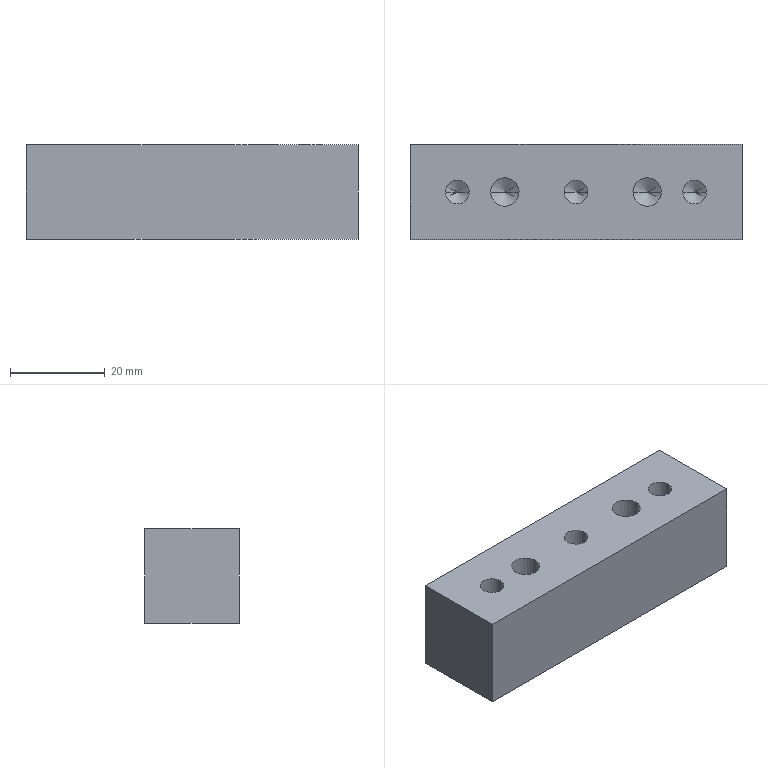Part | STEP file | 11-FG-B08711 | 1 solid | 26 faces | box 70 x 20 x 20 mm | volume 26205 mm3 | cylinder 10 | cone 10 | plane 6 | commonest cylinder face diameters 5 x6 6 x4
STEP:
#1=CARTESIAN_POINT('',(-18.,0.,5.));
#2=VERTEX_POINT('',#1);
#3=CARTESIAN_POINT('',(-12.,0.,5.));
#4=VERTEX_POINT('',#3);
#5=CARTESIAN_POINT('',(-15.,0.,5.));
#6=DIRECTION('',(0.,0.,1.));
#7=DIRECTION('',(1.,0.,0.));
#8=AXIS2_PLACEMENT_3D('',#5,#6,#7);
#9=CIRCLE('',#8,3.);
#10=EDGE_CURVE('',#2,#4,#9,.T.);
#11=ORIENTED_EDGE('',*,*,#10,.F.);
#12=CARTESIAN_POINT('',(-18.,0.,20.));
#13=VERTEX_POINT('',#12);
#14=CARTESIAN_POINT('',(-18.,0.,20.));
#15=DIRECTION('',(0.,0.,1.));
#16=VECTOR('',#15,1000.);
#17=LINE('',#14,#16);
#18=EDGE_CURVE('',#2,#13,#17,.T.);
#19=ORIENTED_EDGE('',*,*,#18,.T.);
#20=CARTESIAN_POINT('',(-12.,0.,20.));
#21=VERTEX_POINT('',#20);
#22=CARTESIAN_POINT('',(-15.,0.,20.));
#23=DIRECTION('',(0.,0.,1.));
#24=DIRECTION('',(1.,0.,0.));
#25=AXIS2_PLACEMENT_3D('',#22,#23,#24);
#26=CIRCLE('',#25,3.);
#27=EDGE_CURVE('',#13,#21,#26,.T.);
#28=ORIENTED_EDGE('',*,*,#27,.T.);
#29=CARTESIAN_POINT('',(-12.,0.,20.));
#30=DIRECTION('',(0.,0.,1.));
#31=VECTOR('',#30,1000.);
#32=LINE('',#29,#31);
#33=EDGE_CURVE('',#4,#21,#32,.T.);
#34=ORIENTED_EDGE('',*,*,#33,.F.);
#35=EDGE_LOOP('',(#11,#19,#28,#34));
#36=FACE_OUTER_BOUND('',#35,.T.);
#37=CARTESIAN_POINT('',(-15.,0.,20.));
#38=DIRECTION('',(0.,0.,1.));
#39=DIRECTION('',(1.,0.,0.));
#40=AXIS2_PLACEMENT_3D('',#37,#38,#39);
#41=CYLINDRICAL_SURFACE('',#40,3.);
#42=ADVANCED_FACE('',(#36),#41,.F.);
#43=CARTESIAN_POINT('',(-15.,0.,3.197));
#44=VERTEX_POINT('',#43);
#45=CARTESIAN_POINT('',(-12.,0.,5.));
#46=DIRECTION('',(0.8572,0.,0.515));
#47=VECTOR('',#46,1000.);
#48=LINE('',#45,#47);
#49=EDGE_CURVE('',#44,#4,#48,.T.);
#50=ORIENTED_EDGE('',*,*,#49,.F.);
#51=CARTESIAN_POINT('',(-18.,0.,5.));
#52=DIRECTION('',(-0.8572,0.,0.515));
#53=VECTOR('',#52,1000.);
#54=LINE('',#51,#53);
#55=EDGE_CURVE('',#44,#2,#54,.T.);
#56=ORIENTED_EDGE('',*,*,#55,.T.);
#57=ORIENTED_EDGE('',*,*,#10,.T.);
#58=EDGE_LOOP('',(#50,#56,#57));
#59=FACE_OUTER_BOUND('',#58,.T.);
#60=CARTESIAN_POINT('',(-15.,0.,5.));
#61=DIRECTION('',(0.,0.,1.));
#62=DIRECTION('',(1.,0.,0.));
#63=AXIS2_PLACEMENT_3D('',#60,#61,#62);
#64=CONICAL_SURFACE('',#63,3.,1.03);
#65=ADVANCED_FACE('',(#59),#64,.F.);
#66=CARTESIAN_POINT('',(12.,0.,5.));
#67=VERTEX_POINT('',#66);
#68=CARTESIAN_POINT('',(18.,0.,5.));
#69=VERTEX_POINT('',#68);
#70=CARTESIAN_POINT('',(15.,0.,5.));
#71=DIRECTION('',(0.,0.,1.));
#72=DIRECTION('',(1.,0.,0.));
#73=AXIS2_PLACEMENT_3D('',#70,#71,#72);
#74=CIRCLE('',#73,3.);
#75=EDGE_CURVE('',#67,#69,#74,.T.);
#76=ORIENTED_EDGE('',*,*,#75,.F.);
#77=CARTESIAN_POINT('',(12.,0.,20.));
#78=VERTEX_POINT('',#77);
#79=CARTESIAN_POINT('',(12.,0.,20.));
#80=DIRECTION('',(0.,0.,1.));
#81=VECTOR('',#80,1000.);
#82=LINE('',#79,#81);
#83=EDGE_CURVE('',#67,#78,#82,.T.);
#84=ORIENTED_EDGE('',*,*,#83,.T.);
#85=CARTESIAN_POINT('',(18.,0.,20.));
#86=VERTEX_POINT('',#85);
#87=CARTESIAN_POINT('',(15.,0.,20.));
#88=DIRECTION('',(0.,0.,1.));
#89=DIRECTION('',(1.,0.,0.));
#90=AXIS2_PLACEMENT_3D('',#87,#88,#89);
#91=CIRCLE('',#90,3.);
#92=EDGE_CURVE('',#78,#86,#91,.T.);
#93=ORIENTED_EDGE('',*,*,#92,.T.);
#94=CARTESIAN_POINT('',(18.,0.,20.));
#95=DIRECTION('',(0.,0.,1.));
#96=VECTOR('',#95,1000.);
#97=LINE('',#94,#96);
#98=EDGE_CURVE('',#69,#86,#97,.T.);
#99=ORIENTED_EDGE('',*,*,#98,.F.);
#100=EDGE_LOOP('',(#76,#84,#93,#99));
#101=FACE_OUTER_BOUND('',#100,.T.);
#102=CARTESIAN_POINT('',(15.,0.,20.));
#103=DIRECTION('',(0.,0.,1.));
#104=DIRECTION('',(1.,0.,0.));
#105=AXIS2_PLACEMENT_3D('',#102,#103,#104);
#106=CYLINDRICAL_SURFACE('',#105,3.);
#107=ADVANCED_FACE('',(#101),#106,.F.);
#108=CARTESIAN_POINT('',(15.,0.,3.197));
#109=VERTEX_POINT('',#108);
#110=CARTESIAN_POINT('',(18.,0.,5.));
#111=DIRECTION('',(0.8572,0.,0.515));
#112=VECTOR('',#111,1000.);
#113=LINE('',#110,#112);
#114=EDGE_CURVE('',#109,#69,#113,.T.);
#115=ORIENTED_EDGE('',*,*,#114,.F.);
#116=CARTESIAN_POINT('',(12.,0.,5.));
#117=DIRECTION('',(-0.8572,0.,0.515));
#118=VECTOR('',#117,1000.);
#119=LINE('',#116,#118);
#120=EDGE_CURVE('',#109,#67,#119,.T.);
#121=ORIENTED_EDGE('',*,*,#120,.T.);
#122=ORIENTED_EDGE('',*,*,#75,.T.);
#123=EDGE_LOOP('',(#115,#121,#122));
#124=FACE_OUTER_BOUND('',#123,.T.);
#125=CARTESIAN_POINT('',(15.,0.,5.));
#126=DIRECTION('',(0.,0.,1.));
#127=DIRECTION('',(1.,0.,0.));
#128=AXIS2_PLACEMENT_3D('',#125,#126,#127);
#129=CONICAL_SURFACE('',#128,3.,1.03);
#130=ADVANCED_FACE('',(#124),#129,.F.);
#131=CARTESIAN_POINT('',(-27.5,0.,5.));
#132=VERTEX_POINT('',#131);
#133=CARTESIAN_POINT('',(-22.5,0.,5.));
#134=VERTEX_POINT('',#133);
#135=CARTESIAN_POINT('',(-25.,0.,5.));
#136=DIRECTION('',(0.,0.,1.));
#137=DIRECTION('',(1.,0.,0.));
#138=AXIS2_PLACEMENT_3D('',#135,#136,#137);
#139=CIRCLE('',#138,2.5);
#140=EDGE_CURVE('',#132,#134,#139,.T.);
#141=ORIENTED_EDGE('',*,*,#140,.F.);
#142=CARTESIAN_POINT('',(-27.5,0.,20.));
#143=VERTEX_POINT('',#142);
#144=CARTESIAN_POINT('',(-27.5,0.,20.));
#145=DIRECTION('',(0.,0.,1.));
#146=VECTOR('',#145,1000.);
#147=LINE('',#144,#146);
#148=EDGE_CURVE('',#132,#143,#147,.T.);
#149=ORIENTED_EDGE('',*,*,#148,.T.);
#150=CARTESIAN_POINT('',(-22.5,0.,20.));
#151=VERTEX_POINT('',#150);
#152=CARTESIAN_POINT('',(-25.,0.,20.));
#153=DIRECTION('',(0.,0.,1.));
#154=DIRECTION('',(1.,0.,0.));
#155=AXIS2_PLACEMENT_3D('',#152,#153,#154);
#156=CIRCLE('',#155,2.5);
#157=EDGE_CURVE('',#143,#151,#156,.T.);
#158=ORIENTED_EDGE('',*,*,#157,.T.);
#159=CARTESIAN_POINT('',(-22.5,0.,20.));
#160=DIRECTION('',(0.,0.,1.));
#161=VECTOR('',#160,1000.);
#162=LINE('',#159,#161);
#163=EDGE_CURVE('',#134,#151,#162,.T.);
#164=ORIENTED_EDGE('',*,*,#163,.F.);
#165=EDGE_LOOP('',(#141,#149,#158,#164));
#166=FACE_OUTER_BOUND('',#165,.T.);
#167=CARTESIAN_POINT('',(-25.,0.,20.));
#168=DIRECTION('',(0.,0.,1.));
#169=DIRECTION('',(1.,0.,0.));
#170=AXIS2_PLACEMENT_3D('',#167,#168,#169);
#171=CYLINDRICAL_SURFACE('',#170,2.5);
#172=ADVANCED_FACE('',(#166),#171,.F.);
#173=CARTESIAN_POINT('',(-25.,0.,3.498));
#174=VERTEX_POINT('',#173);
#175=CARTESIAN_POINT('',(-22.5,0.,5.));
#176=DIRECTION('',(0.8572,0.,0.515));
#177=VECTOR('',#176,1000.);
#178=LINE('',#175,#177);
#179=EDGE_CURVE('',#174,#134,#178,.T.);
#180=ORIENTED_EDGE('',*,*,#179,.F.);
#181=CARTESIAN_POINT('',(-27.5,0.,5.));
#182=DIRECTION('',(-0.8572,0.,0.515));
#183=VECTOR('',#182,1000.);
#184=LINE('',#181,#183);
#185=EDGE_CURVE('',#174,#132,#184,.T.);
#186=ORIENTED_EDGE('',*,*,#185,.T.);
#187=ORIENTED_EDGE('',*,*,#140,.T.);
#188=EDGE_LOOP('',(#180,#186,#187));
#189=FACE_OUTER_BOUND('',#188,.T.);
#190=CARTESIAN_POINT('',(-25.,0.,5.));
#191=DIRECTION('',(0.,0.,1.));
#192=DIRECTION('',(1.,0.,0.));
#193=AXIS2_PLACEMENT_3D('',#190,#191,#192);
#194=CONICAL_SURFACE('',#193,2.5,1.03);
#195=ADVANCED_FACE('',(#189),#194,.F.);
#196=CARTESIAN_POINT('',(-2.5,0.,5.));
#197=VERTEX_POINT('',#196);
#198=CARTESIAN_POINT('',(2.5,0.,5.));
#199=VERTEX_POINT('',#198);
#200=CARTESIAN_POINT('',(0.,0.,5.));
#201=DIRECTION('',(0.,0.,1.));
#202=DIRECTION('',(1.,0.,0.));
#203=AXIS2_PLACEMENT_3D('',#200,#201,#202);
#204=CIRCLE('',#203,2.5);
#205=EDGE_CURVE('',#197,#199,#204,.T.);
#206=ORIENTED_EDGE('',*,*,#205,.F.);
#207=CARTESIAN_POINT('',(-2.5,0.,20.));
#208=VERTEX_POINT('',#207);
#209=CARTESIAN_POINT('',(-2.5,0.,20.));
#210=DIRECTION('',(0.,0.,1.));
#211=VECTOR('',#210,1000.);
#212=LINE('',#209,#211);
#213=EDGE_CURVE('',#197,#208,#212,.T.);
#214=ORIENTED_EDGE('',*,*,#213,.T.);
#215=CARTESIAN_POINT('',(2.5,0.,20.));
#216=VERTEX_POINT('',#215);
#217=CARTESIAN_POINT('',(0.,0.,20.));
#218=DIRECTION('',(0.,0.,1.));
#219=DIRECTION('',(1.,0.,0.));
#220=AXIS2_PLACEMENT_3D('',#217,#218,#219);
#221=CIRCLE('',#220,2.5);
#222=EDGE_CURVE('',#208,#216,#221,.T.);
#223=ORIENTED_EDGE('',*,*,#222,.T.);
#224=CARTESIAN_POINT('',(2.5,0.,20.));
#225=DIRECTION('',(0.,0.,1.));
#226=VECTOR('',#225,1000.);
#227=LINE('',#224,#226);
#228=EDGE_CURVE('',#199,#216,#227,.T.);
#229=ORIENTED_EDGE('',*,*,#228,.F.);
#230=EDGE_LOOP('',(#206,#214,#223,#229));
#231=FACE_OUTER_BOUND('',#230,.T.);
#232=CARTESIAN_POINT('',(0.,0.,20.));
#233=DIRECTION('',(0.,0.,1.));
#234=DIRECTION('',(1.,0.,0.));
#235=AXIS2_PLACEMENT_3D('',#232,#233,#234);
#236=CYLINDRICAL_SURFACE('',#235,2.5);
#237=ADVANCED_FACE('',(#231),#236,.F.);
#238=CARTESIAN_POINT('',(0.,0.,3.498));
#239=VERTEX_POINT('',#238);
#240=CARTESIAN_POINT('',(2.5,0.,5.));
#241=DIRECTION('',(0.8572,0.,0.515));
#242=VECTOR('',#241,1000.);
#243=LINE('',#240,#242);
#244=EDGE_CURVE('',#239,#199,#243,.T.);
#245=ORIENTED_EDGE('',*,*,#244,.F.);
#246=CARTESIAN_POINT('',(-2.5,0.,5.));
#247=DIRECTION('',(-0.8572,0.,0.515));
#248=VECTOR('',#247,1000.);
#249=LINE('',#246,#248);
#250=EDGE_CURVE('',#239,#197,#249,.T.);
#251=ORIENTED_EDGE('',*,*,#250,.T.);
#252=ORIENTED_EDGE('',*,*,#205,.T.);
#253=EDGE_LOOP('',(#245,#251,#252));
#254=FACE_OUTER_BOUND('',#253,.T.);
#255=CARTESIAN_POINT('',(0.,0.,5.));
#256=DIRECTION('',(0.,0.,1.));
#257=DIRECTION('',(1.,0.,0.));
#258=AXIS2_PLACEMENT_3D('',#255,#256,#257);
#259=CONICAL_SURFACE('',#258,2.5,1.03);
#260=ADVANCED_FACE('',(#254),#259,.F.);
#261=CARTESIAN_POINT('',(22.5,0.,5.));
#262=VERTEX_POINT('',#261);
#263=CARTESIAN_POINT('',(27.5,0.,5.));
#264=VERTEX_POINT('',#263);
#265=CARTESIAN_POINT('',(25.,0.,5.));
#266=DIRECTION('',(0.,0.,1.));
#267=DIRECTION('',(1.,0.,0.));
#268=AXIS2_PLACEMENT_3D('',#265,#266,#267);
#269=CIRCLE('',#268,2.5);
#270=EDGE_CURVE('',#262,#264,#269,.T.);
#271=ORIENTED_EDGE('',*,*,#270,.F.);
#272=CARTESIAN_POINT('',(22.5,0.,20.));
#273=VERTEX_POINT('',#272);
#274=CARTESIAN_POINT('',(22.5,0.,20.));
#275=DIRECTION('',(0.,0.,1.));
#276=VECTOR('',#275,1000.);
#277=LINE('',#274,#276);
#278=EDGE_CURVE('',#262,#273,#277,.T.);
#279=ORIENTED_EDGE('',*,*,#278,.T.);
#280=CARTESIAN_POINT('',(27.5,0.,20.));
#281=VERTEX_POINT('',#280);
#282=CARTESIAN_POINT('',(25.,0.,20.));
#283=DIRECTION('',(0.,0.,1.));
#284=DIRECTION('',(1.,0.,0.));
#285=AXIS2_PLACEMENT_3D('',#282,#283,#284);
#286=CIRCLE('',#285,2.5);
#287=EDGE_CURVE('',#273,#281,#286,.T.);
#288=ORIENTED_EDGE('',*,*,#287,.T.);
#289=CARTESIAN_POINT('',(27.5,0.,20.));
#290=DIRECTION('',(0.,0.,1.));
#291=VECTOR('',#290,1000.);
#292=LINE('',#289,#291);
#293=EDGE_CURVE('',#264,#281,#292,.T.);
#294=ORIENTED_EDGE('',*,*,#293,.F.);
#295=EDGE_LOOP('',(#271,#279,#288,#294));
#296=FACE_OUTER_BOUND('',#295,.T.);
#297=CARTESIAN_POINT('',(25.,0.,20.));
#298=DIRECTION('',(0.,0.,1.));
#299=DIRECTION('',(1.,0.,0.));
#300=AXIS2_PLACEMENT_3D('',#297,#298,#299);
#301=CYLINDRICAL_SURFACE('',#300,2.5);
#302=ADVANCED_FACE('',(#296),#301,.F.);
#303=CARTESIAN_POINT('',(25.,0.,3.498));
#304=VERTEX_POINT('',#303);
#305=CARTESIAN_POINT('',(27.5,0.,5.));
#306=DIRECTION('',(0.8572,0.,0.515));
#307=VECTOR('',#306,1000.);
#308=LINE('',#305,#307);
#309=EDGE_CURVE('',#304,#264,#308,.T.);
#310=ORIENTED_EDGE('',*,*,#309,.F.);
#311=CARTESIAN_POINT('',(22.5,0.,5.));
#312=DIRECTION('',(-0.8572,0.,0.515));
#313=VECTOR('',#312,1000.);
#314=LINE('',#311,#313);
#315=EDGE_CURVE('',#304,#262,#314,.T.);
#316=ORIENTED_EDGE('',*,*,#315,.T.);
#317=ORIENTED_EDGE('',*,*,#270,.T.);
#318=EDGE_LOOP('',(#310,#316,#317));
#319=FACE_OUTER_BOUND('',#318,.T.);
#320=CARTESIAN_POINT('',(25.,0.,5.));
#321=DIRECTION('',(0.,0.,1.));
#322=DIRECTION('',(1.,0.,0.));
#323=AXIS2_PLACEMENT_3D('',#320,#321,#322);
#324=CONICAL_SURFACE('',#323,2.5,1.03);
#325=ADVANCED_FACE('',(#319),#324,.F.);
#326=CARTESIAN_POINT('',(35.,-10.,0.));
#327=VERTEX_POINT('',#326);
#328=CARTESIAN_POINT('',(35.,10.,0.));
#329=VERTEX_POINT('',#328);
#330=CARTESIAN_POINT('',(35.,10.,0.));
#331=DIRECTION('',(0.,1.,0.));
#332=VECTOR('',#331,1000.);
#333=LINE('',#330,#332);
#334=EDGE_CURVE('',#327,#329,#333,.T.);
#335=ORIENTED_EDGE('',*,*,#334,.T.);
#336=CARTESIAN_POINT('',(35.,10.,20.));
#337=VERTEX_POINT('',#336);
#338=CARTESIAN_POINT('',(35.,10.,20.));
#339=DIRECTION('',(0.,0.,-1.));
#340=VECTOR('',#339,1000.);
#341=LINE('',#338,#340);
#342=EDGE_CURVE('',#337,#329,#341,.T.);
#343=ORIENTED_EDGE('',*,*,#342,.F.);
#344=CARTESIAN_POINT('',(35.,-10.,20.));
#345=VERTEX_POINT('',#344);
#346=CARTESIAN_POINT('',(35.,10.,20.));
#347=DIRECTION('',(0.,1.,0.));
#348=VECTOR('',#347,1000.);
#349=LINE('',#346,#348);
#350=EDGE_CURVE('',#345,#337,#349,.T.);
#351=ORIENTED_EDGE('',*,*,#350,.F.);
#352=CARTESIAN_POINT('',(35.,-10.,20.));
#353=DIRECTION('',(0.,0.,-1.));
#354=VECTOR('',#353,1000.);
#355=LINE('',#352,#354);
#356=EDGE_CURVE('',#345,#327,#355,.T.);
#357=ORIENTED_EDGE('',*,*,#356,.T.);
#358=EDGE_LOOP('',(#335,#343,#351,#357));
#359=FACE_OUTER_BOUND('',#358,.T.);
#360=CARTESIAN_POINT('',(35.,10.,20.));
#361=DIRECTION('',(-1.,0.,0.));
#362=DIRECTION('',(0.,-1.,0.));
#363=AXIS2_PLACEMENT_3D('',#360,#361,#362);
#364=PLANE('',#363);
#365=ADVANCED_FACE('',(#359),#364,.F.);
#366=CARTESIAN_POINT('',(-35.,10.,0.));
#367=VERTEX_POINT('',#366);
#368=CARTESIAN_POINT('',(-35.,10.,0.));
#369=DIRECTION('',(-1.,0.,0.));
#370=VECTOR('',#369,1000.);
#371=LINE('',#368,#370);
#372=EDGE_CURVE('',#329,#367,#371,.T.);
#373=ORIENTED_EDGE('',*,*,#372,.T.);
#374=CARTESIAN_POINT('',(-35.,10.,20.));
#375=VERTEX_POINT('',#374);
#376=CARTESIAN_POINT('',(-35.,10.,20.));
#377=DIRECTION('',(0.,0.,-1.));
#378=VECTOR('',#377,1000.);
#379=LINE('',#376,#378);
#380=EDGE_CURVE('',#375,#367,#379,.T.);
#381=ORIENTED_EDGE('',*,*,#380,.F.);
#382=CARTESIAN_POINT('',(-35.,10.,20.));
#383=DIRECTION('',(-1.,0.,0.));
#384=VECTOR('',#383,1000.);
#385=LINE('',#382,#384);
#386=EDGE_CURVE('',#337,#375,#385,.T.);
#387=ORIENTED_EDGE('',*,*,#386,.F.);
#388=ORIENTED_EDGE('',*,*,#342,.T.);
#389=EDGE_LOOP('',(#373,#381,#387,#388));
#390=FACE_OUTER_BOUND('',#389,.T.);
#391=CARTESIAN_POINT('',(-35.,10.,20.));
#392=DIRECTION('',(0.,-1.,0.));
#393=DIRECTION('',(0.,0.,-1.));
#394=AXIS2_PLACEMENT_3D('',#391,#392,#393);
#395=PLANE('',#394);
#396=ADVANCED_FACE('',(#390),#395,.F.);
#397=CARTESIAN_POINT('',(-35.,-10.,0.));
#398=VERTEX_POINT('',#397);
#399=CARTESIAN_POINT('',(-35.,10.,0.));
#400=DIRECTION('',(0.,-1.,0.));
#401=VECTOR('',#400,1000.);
#402=LINE('',#399,#401);
#403=EDGE_CURVE('',#367,#398,#402,.T.);
#404=ORIENTED_EDGE('',*,*,#403,.T.);
#405=CARTESIAN_POINT('',(-35.,-10.,20.));
#406=VERTEX_POINT('',#405);
#407=CARTESIAN_POINT('',(-35.,-10.,20.));
#408=DIRECTION('',(0.,0.,-1.));
#409=VECTOR('',#408,1000.);
#410=LINE('',#407,#409);
#411=EDGE_CURVE('',#406,#398,#410,.T.);
#412=ORIENTED_EDGE('',*,*,#411,.F.);
#413=CARTESIAN_POINT('',(-35.,10.,20.));
#414=DIRECTION('',(0.,-1.,0.));
#415=VECTOR('',#414,1000.);
#416=LINE('',#413,#415);
#417=EDGE_CURVE('',#375,#406,#416,.T.);
#418=ORIENTED_EDGE('',*,*,#417,.F.);
#419=ORIENTED_EDGE('',*,*,#380,.T.);
#420=EDGE_LOOP('',(#404,#412,#418,#419));
#421=FACE_OUTER_BOUND('',#420,.T.);
#422=CARTESIAN_POINT('',(-35.,10.,20.));
#423=DIRECTION('',(1.,0.,0.));
#424=DIRECTION('',(0.,1.,0.));
#425=AXIS2_PLACEMENT_3D('',#422,#423,#424);
#426=PLANE('',#425);
#427=ADVANCED_FACE('',(#421),#426,.F.);
#428=CARTESIAN_POINT('',(-35.,-10.,0.));
#429=DIRECTION('',(1.,0.,0.));
#430=VECTOR('',#429,1000.);
#431=LINE('',#428,#430);
#432=EDGE_CURVE('',#398,#327,#431,.T.);
#433=ORIENTED_EDGE('',*,*,#432,.T.);
#434=ORIENTED_EDGE('',*,*,#356,.F.);
#435=CARTESIAN_POINT('',(-35.,-10.,20.));
#436=DIRECTION('',(1.,0.,0.));
#437=VECTOR('',#436,1000.);
#438=LINE('',#435,#437);
#439=EDGE_CURVE('',#406,#345,#438,.T.);
#440=ORIENTED_EDGE('',*,*,#439,.F.);
#441=ORIENTED_EDGE('',*,*,#411,.T.);
#442=EDGE_LOOP('',(#433,#434,#440,#441));
#443=FACE_OUTER_BOUND('',#442,.T.);
#444=CARTESIAN_POINT('',(-35.,-10.,20.));
#445=DIRECTION('',(0.,1.,0.));
#446=DIRECTION('',(0.,0.,1.));
#447=AXIS2_PLACEMENT_3D('',#444,#445,#446);
#448=PLANE('',#447);
#449=ADVANCED_FACE('',(#443),#448,.F.);
#450=CARTESIAN_POINT('',(-15.,0.,20.));
#451=DIRECTION('',(0.,0.,1.));
#452=DIRECTION('',(1.,0.,0.));
#453=AXIS2_PLACEMENT_3D('',#450,#451,#452);
#454=CIRCLE('',#453,3.);
#455=EDGE_CURVE('',#21,#13,#454,.T.);
#456=ORIENTED_EDGE('',*,*,#455,.F.);
#457=ORIENTED_EDGE('',*,*,#27,.F.);
#458=EDGE_LOOP('',(#456,#457));
#459=FACE_BOUND('',#458,.T.);
#460=CARTESIAN_POINT('',(15.,0.,20.));
#461=DIRECTION('',(0.,0.,1.));
#462=DIRECTION('',(1.,0.,0.));
#463=AXIS2_PLACEMENT_3D('',#460,#461,#462);
#464=CIRCLE('',#463,3.);
#465=EDGE_CURVE('',#86,#78,#464,.T.);
#466=ORIENTED_EDGE('',*,*,#465,.F.);
#467=ORIENTED_EDGE('',*,*,#92,.F.);
#468=EDGE_LOOP('',(#466,#467));
#469=FACE_BOUND('',#468,.T.);
#470=CARTESIAN_POINT('',(-25.,0.,20.));
#471=DIRECTION('',(0.,0.,1.));
#472=DIRECTION('',(1.,0.,0.));
#473=AXIS2_PLACEMENT_3D('',#470,#471,#472);
#474=CIRCLE('',#473,2.5);
#475=EDGE_CURVE('',#151,#143,#474,.T.);
#476=ORIENTED_EDGE('',*,*,#475,.F.);
#477=ORIENTED_EDGE('',*,*,#157,.F.);
#478=EDGE_LOOP('',(#476,#477));
#479=FACE_BOUND('',#478,.T.);
#480=CARTESIAN_POINT('',(0.,0.,20.));
#481=DIRECTION('',(0.,0.,1.));
#482=DIRECTION('',(1.,0.,0.));
#483=AXIS2_PLACEMENT_3D('',#480,#481,#482);
#484=CIRCLE('',#483,2.5);
#485=EDGE_CURVE('',#216,#208,#484,.T.);
#486=ORIENTED_EDGE('',*,*,#485,.F.);
#487=ORIENTED_EDGE('',*,*,#222,.F.);
#488=EDGE_LOOP('',(#486,#487));
#489=FACE_BOUND('',#488,.T.);
#490=CARTESIAN_POINT('',(25.,0.,20.));
#491=DIRECTION('',(0.,0.,1.));
#492=DIRECTION('',(1.,0.,0.));
#493=AXIS2_PLACEMENT_3D('',#490,#491,#492);
#494=CIRCLE('',#493,2.5);
#495=EDGE_CURVE('',#281,#273,#494,.T.);
#496=ORIENTED_EDGE('',*,*,#495,.F.);
#497=ORIENTED_EDGE('',*,*,#287,.F.);
#498=EDGE_LOOP('',(#496,#497));
#499=FACE_BOUND('',#498,.T.);
#500=ORIENTED_EDGE('',*,*,#350,.T.);
#501=ORIENTED_EDGE('',*,*,#386,.T.);
#502=ORIENTED_EDGE('',*,*,#417,.T.);
#503=ORIENTED_EDGE('',*,*,#439,.T.);
#504=EDGE_LOOP('',(#500,#501,#502,#503));
#505=FACE_OUTER_BOUND('',#504,.T.);
#506=CARTESIAN_POINT('',(0.,0.,20.));
#507=DIRECTION('',(0.,0.,1.));
#508=DIRECTION('',(1.,0.,0.));
#509=AXIS2_PLACEMENT_3D('',#506,#507,#508);
#510=PLANE('',#509);
#511=ADVANCED_FACE('',(#459,#469,#479,#489,#499,#505),#510,.T.);
#512=ORIENTED_EDGE('',*,*,#334,.F.);
#513=ORIENTED_EDGE('',*,*,#432,.F.);
#514=ORIENTED_EDGE('',*,*,#403,.F.);
#515=ORIENTED_EDGE('',*,*,#372,.F.);
#516=EDGE_LOOP('',(#512,#513,#514,#515));
#517=FACE_OUTER_BOUND('',#516,.T.);
#518=CARTESIAN_POINT('',(0.,0.,0.));
#519=DIRECTION('',(0.,0.,1.));
#520=DIRECTION('',(1.,0.,0.));
#521=AXIS2_PLACEMENT_3D('',#518,#519,#520);
#522=PLANE('',#521);
#523=ADVANCED_FACE('',(#517),#522,.F.);
#524=ORIENTED_EDGE('',*,*,#315,.F.);
#525=ORIENTED_EDGE('',*,*,#309,.T.);
#526=CARTESIAN_POINT('',(25.,0.,5.));
#527=DIRECTION('',(0.,0.,1.));
#528=DIRECTION('',(1.,0.,0.));
#529=AXIS2_PLACEMENT_3D('',#526,#527,#528);
#530=CIRCLE('',#529,2.5);
#531=EDGE_CURVE('',#264,#262,#530,.T.);
#532=ORIENTED_EDGE('',*,*,#531,.T.);
#533=EDGE_LOOP('',(#524,#525,#532));
#534=FACE_OUTER_BOUND('',#533,.T.);
#535=CARTESIAN_POINT('',(25.,0.,5.));
#536=DIRECTION('',(0.,0.,1.));
#537=DIRECTION('',(1.,0.,0.));
#538=AXIS2_PLACEMENT_3D('',#535,#536,#537);
#539=CONICAL_SURFACE('',#538,2.5,1.03);
#540=ADVANCED_FACE('',(#534),#539,.F.);
#541=ORIENTED_EDGE('',*,*,#278,.F.);
#542=ORIENTED_EDGE('',*,*,#531,.F.);
#543=ORIENTED_EDGE('',*,*,#293,.T.);
#544=ORIENTED_EDGE('',*,*,#495,.T.);
#545=EDGE_LOOP('',(#541,#542,#543,#544));
#546=FACE_OUTER_BOUND('',#545,.T.);
#547=CARTESIAN_POINT('',(25.,0.,20.));
#548=DIRECTION('',(0.,0.,1.));
#549=DIRECTION('',(1.,0.,0.));
#550=AXIS2_PLACEMENT_3D('',#547,#548,#549);
#551=CYLINDRICAL_SURFACE('',#550,2.5);
#552=ADVANCED_FACE('',(#546),#551,.F.);
#553=ORIENTED_EDGE('',*,*,#250,.F.);
#554=ORIENTED_EDGE('',*,*,#244,.T.);
#555=CARTESIAN_POINT('',(0.,0.,5.));
#556=DIRECTION('',(0.,0.,1.));
#557=DIRECTION('',(1.,0.,0.));
#558=AXIS2_PLACEMENT_3D('',#555,#556,#557);
#559=CIRCLE('',#558,2.5);
#560=EDGE_CURVE('',#199,#197,#559,.T.);
#561=ORIENTED_EDGE('',*,*,#560,.T.);
#562=EDGE_LOOP('',(#553,#554,#561));
#563=FACE_OUTER_BOUND('',#562,.T.);
#564=CARTESIAN_POINT('',(0.,0.,5.));
#565=DIRECTION('',(0.,0.,1.));
#566=DIRECTION('',(1.,0.,0.));
#567=AXIS2_PLACEMENT_3D('',#564,#565,#566);
#568=CONICAL_SURFACE('',#567,2.5,1.03);
#569=ADVANCED_FACE('',(#563),#568,.F.);
#570=ORIENTED_EDGE('',*,*,#213,.F.);
#571=ORIENTED_EDGE('',*,*,#560,.F.);
#572=ORIENTED_EDGE('',*,*,#228,.T.);
#573=ORIENTED_EDGE('',*,*,#485,.T.);
#574=EDGE_LOOP('',(#570,#571,#572,#573));
#575=FACE_OUTER_BOUND('',#574,.T.);
#576=CARTESIAN_POINT('',(0.,0.,20.));
#577=DIRECTION('',(0.,0.,1.));
#578=DIRECTION('',(1.,0.,0.));
#579=AXIS2_PLACEMENT_3D('',#576,#577,#578);
#580=CYLINDRICAL_SURFACE('',#579,2.5);
#581=ADVANCED_FACE('',(#575),#580,.F.);
#582=ORIENTED_EDGE('',*,*,#185,.F.);
#583=ORIENTED_EDGE('',*,*,#179,.T.);
#584=CARTESIAN_POINT('',(-25.,0.,5.));
#585=DIRECTION('',(0.,0.,1.));
#586=DIRECTION('',(1.,0.,0.));
#587=AXIS2_PLACEMENT_3D('',#584,#585,#586);
#588=CIRCLE('',#587,2.5);
#589=EDGE_CURVE('',#134,#132,#588,.T.);
#590=ORIENTED_EDGE('',*,*,#589,.T.);
#591=EDGE_LOOP('',(#582,#583,#590));
#592=FACE_OUTER_BOUND('',#591,.T.);
#593=CARTESIAN_POINT('',(-25.,0.,5.));
#594=DIRECTION('',(0.,0.,1.));
#595=DIRECTION('',(1.,0.,0.));
#596=AXIS2_PLACEMENT_3D('',#593,#594,#595);
#597=CONICAL_SURFACE('',#596,2.5,1.03);
#598=ADVANCED_FACE('',(#592),#597,.F.);
#599=ORIENTED_EDGE('',*,*,#148,.F.);
#600=ORIENTED_EDGE('',*,*,#589,.F.);
#601=ORIENTED_EDGE('',*,*,#163,.T.);
#602=ORIENTED_EDGE('',*,*,#475,.T.);
#603=EDGE_LOOP('',(#599,#600,#601,#602));
#604=FACE_OUTER_BOUND('',#603,.T.);
#605=CARTESIAN_POINT('',(-25.,0.,20.));
#606=DIRECTION('',(0.,0.,1.));
#607=DIRECTION('',(1.,0.,0.));
#608=AXIS2_PLACEMENT_3D('',#605,#606,#607);
#609=CYLINDRICAL_SURFACE('',#608,2.5);
#610=ADVANCED_FACE('',(#604),#609,.F.);
#611=ORIENTED_EDGE('',*,*,#120,.F.);
#612=ORIENTED_EDGE('',*,*,#114,.T.);
#613=CARTESIAN_POINT('',(15.,0.,5.));
#614=DIRECTION('',(0.,0.,1.));
#615=DIRECTION('',(1.,0.,0.));
#616=AXIS2_PLACEMENT_3D('',#613,#614,#615);
#617=CIRCLE('',#616,3.);
#618=EDGE_CURVE('',#69,#67,#617,.T.);
#619=ORIENTED_EDGE('',*,*,#618,.T.);
#620=EDGE_LOOP('',(#611,#612,#619));
#621=FACE_OUTER_BOUND('',#620,.T.);
#622=CARTESIAN_POINT('',(15.,0.,5.));
#623=DIRECTION('',(0.,0.,1.));
#624=DIRECTION('',(1.,0.,0.));
#625=AXIS2_PLACEMENT_3D('',#622,#623,#624);
#626=CONICAL_SURFACE('',#625,3.,1.03);
#627=ADVANCED_FACE('',(#621),#626,.F.);
#628=ORIENTED_EDGE('',*,*,#83,.F.);
#629=ORIENTED_EDGE('',*,*,#618,.F.);
#630=ORIENTED_EDGE('',*,*,#98,.T.);
#631=ORIENTED_EDGE('',*,*,#465,.T.);
#632=EDGE_LOOP('',(#628,#629,#630,#631));
#633=FACE_OUTER_BOUND('',#632,.T.);
#634=CARTESIAN_POINT('',(15.,0.,20.));
#635=DIRECTION('',(0.,0.,1.));
#636=DIRECTION('',(1.,0.,0.));
#637=AXIS2_PLACEMENT_3D('',#634,#635,#636);
#638=CYLINDRICAL_SURFACE('',#637,3.);
#639=ADVANCED_FACE('',(#633),#638,.F.);
#640=ORIENTED_EDGE('',*,*,#55,.F.);
#641=ORIENTED_EDGE('',*,*,#49,.T.);
#642=CARTESIAN_POINT('',(-15.,0.,5.));
#643=DIRECTION('',(0.,0.,1.));
#644=DIRECTION('',(1.,0.,0.));
#645=AXIS2_PLACEMENT_3D('',#642,#643,#644);
#646=CIRCLE('',#645,3.);
#647=EDGE_CURVE('',#4,#2,#646,.T.);
#648=ORIENTED_EDGE('',*,*,#647,.T.);
#649=EDGE_LOOP('',(#640,#641,#648));
#650=FACE_OUTER_BOUND('',#649,.T.);
#651=CARTESIAN_POINT('',(-15.,0.,5.));
#652=DIRECTION('',(0.,0.,1.));
#653=DIRECTION('',(1.,0.,0.));
#654=AXIS2_PLACEMENT_3D('',#651,#652,#653);
#655=CONICAL_SURFACE('',#654,3.,1.03);
#656=ADVANCED_FACE('',(#650),#655,.F.);
#657=ORIENTED_EDGE('',*,*,#18,.F.);
#658=ORIENTED_EDGE('',*,*,#647,.F.);
#659=ORIENTED_EDGE('',*,*,#33,.T.);
#660=ORIENTED_EDGE('',*,*,#455,.T.);
#661=EDGE_LOOP('',(#657,#658,#659,#660));
#662=FACE_OUTER_BOUND('',#661,.T.);
#663=CARTESIAN_POINT('',(-15.,0.,20.));
#664=DIRECTION('',(0.,0.,1.));
#665=DIRECTION('',(1.,0.,0.));
#666=AXIS2_PLACEMENT_3D('',#663,#664,#665);
#667=CYLINDRICAL_SURFACE('',#666,3.);
#668=ADVANCED_FACE('',(#662),#667,.F.);
#669=CLOSED_SHELL('',(#42,#65,#107,#130,#172,#195,#237,#260,#302,#325,#365,#396,#427,#449,#511,#523,#540,#552,#569,#581,#598,#610,#627,#639,#656,#668));
#670=MANIFOLD_SOLID_BREP('',#669);
#671=CARTESIAN_POINT('',(0.,0.,0.));
#672=DIRECTION('',(0.,0.,1.));
#673=DIRECTION('',(1.,0.,0.));
#674=AXIS2_PLACEMENT_3D('',#671,#672,#673);
#675=(LENGTH_UNIT()NAMED_UNIT(*)SI_UNIT(.MILLI.,.METRE.));
#676=UNCERTAINTY_MEASURE_WITH_UNIT(LENGTH_MEASURE(0.00001),#675,'','');
#677=(NAMED_UNIT(*)PLANE_ANGLE_UNIT()SI_UNIT($,.RADIAN.));
#678=(NAMED_UNIT(*)SI_UNIT($,.STERADIAN.)SOLID_ANGLE_UNIT());
#679=(GEOMETRIC_REPRESENTATION_CONTEXT(3)GLOBAL_UNCERTAINTY_ASSIGNED_CONTEXT((#676))GLOBAL_UNIT_ASSIGNED_CONTEXT((#675,#677,#678))REPRESENTATION_CONTEXT('',''));
#680=ADVANCED_BREP_SHAPE_REPRESENTATION('',(#670,#674),#679);